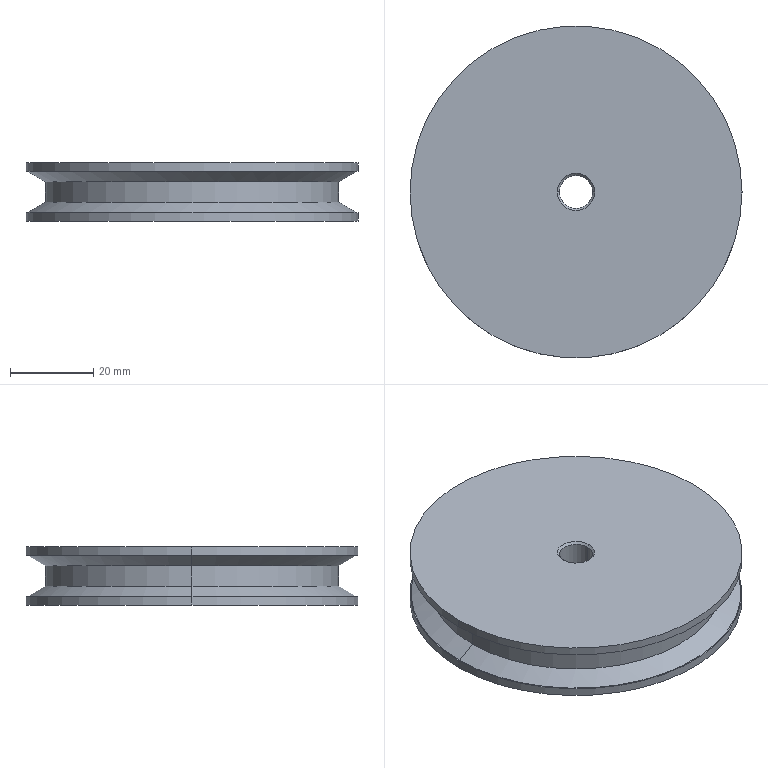Part | SolidWorks | features Chamfer 1, Extrusion 1, RevCut 1 | 1 solid | 20 faces | box 80 x 80 x 14 mm | volume 61206 mm3 | cone 8 | cylinder 8 | plane 4 | commonest cylinder face diameters 80 x4 8 x2 70.651 x2
STEP:
#1=CARTESIAN_POINT('',(4.,0.,-6.5));
#2=VERTEX_POINT('',#1);
#3=CARTESIAN_POINT('',(-4.,0.,-6.5));
#4=VERTEX_POINT('',#3);
#5=CARTESIAN_POINT('',(0.,0.,-6.5));
#6=DIRECTION('',(0.,0.,-1.));
#7=DIRECTION('',(1.,0.,0.));
#8=AXIS2_PLACEMENT_3D('',#5,#6,#7);
#9=CIRCLE('',#8,4.);
#10=EDGE_CURVE('',#2,#4,#9,.T.);
#11=ORIENTED_EDGE('',*,*,#10,.F.);
#12=CARTESIAN_POINT('',(4.5,0.,-7.));
#13=VERTEX_POINT('',#12);
#14=CARTESIAN_POINT('',(4.5,0.,-7.));
#15=DIRECTION('',(0.7071,0.,-0.7071));
#16=VECTOR('',#15,1000.);
#17=LINE('',#14,#16);
#18=EDGE_CURVE('',#2,#13,#17,.T.);
#19=ORIENTED_EDGE('',*,*,#18,.T.);
#20=CARTESIAN_POINT('',(-4.5,0.,-7.));
#21=VERTEX_POINT('',#20);
#22=CARTESIAN_POINT('',(0.,0.,-7.));
#23=DIRECTION('',(0.,0.,1.));
#24=DIRECTION('',(1.,0.,0.));
#25=AXIS2_PLACEMENT_3D('',#22,#23,#24);
#26=CIRCLE('',#25,4.5);
#27=EDGE_CURVE('',#21,#13,#26,.T.);
#28=ORIENTED_EDGE('',*,*,#27,.F.);
#29=CARTESIAN_POINT('',(-4.5,0.,-7.));
#30=DIRECTION('',(-0.7071,0.,-0.7071));
#31=VECTOR('',#30,1000.);
#32=LINE('',#29,#31);
#33=EDGE_CURVE('',#4,#21,#32,.T.);
#34=ORIENTED_EDGE('',*,*,#33,.F.);
#35=EDGE_LOOP('',(#11,#19,#28,#34));
#36=FACE_OUTER_BOUND('',#35,.T.);
#37=CARTESIAN_POINT('',(0.,0.,-7.));
#38=DIRECTION('',(0.,0.,-1.));
#39=DIRECTION('',(-1.,0.,0.));
#40=AXIS2_PLACEMENT_3D('',#37,#38,#39);
#41=CONICAL_SURFACE('',#40,4.5,0.7854);
#42=ADVANCED_FACE('',(#36),#41,.F.);
#43=CARTESIAN_POINT('',(-4.,0.,6.5));
#44=VERTEX_POINT('',#43);
#45=CARTESIAN_POINT('',(4.,0.,6.5));
#46=VERTEX_POINT('',#45);
#47=CARTESIAN_POINT('',(0.,0.,6.5));
#48=DIRECTION('',(0.,0.,1.));
#49=DIRECTION('',(1.,0.,0.));
#50=AXIS2_PLACEMENT_3D('',#47,#48,#49);
#51=CIRCLE('',#50,4.);
#52=EDGE_CURVE('',#44,#46,#51,.T.);
#53=ORIENTED_EDGE('',*,*,#52,.F.);
#54=CARTESIAN_POINT('',(-4.5,0.,7.));
#55=VERTEX_POINT('',#54);
#56=CARTESIAN_POINT('',(-4.,0.,6.5));
#57=DIRECTION('',(-0.7071,0.,0.7071));
#58=VECTOR('',#57,1000.);
#59=LINE('',#56,#58);
#60=EDGE_CURVE('',#44,#55,#59,.T.);
#61=ORIENTED_EDGE('',*,*,#60,.T.);
#62=CARTESIAN_POINT('',(4.5,0.,7.));
#63=VERTEX_POINT('',#62);
#64=CARTESIAN_POINT('',(0.,0.,7.));
#65=DIRECTION('',(0.,0.,-1.));
#66=DIRECTION('',(1.,0.,0.));
#67=AXIS2_PLACEMENT_3D('',#64,#65,#66);
#68=CIRCLE('',#67,4.5);
#69=EDGE_CURVE('',#63,#55,#68,.T.);
#70=ORIENTED_EDGE('',*,*,#69,.F.);
#71=CARTESIAN_POINT('',(4.,0.,6.5));
#72=DIRECTION('',(0.7071,0.,0.7071));
#73=VECTOR('',#72,1000.);
#74=LINE('',#71,#73);
#75=EDGE_CURVE('',#46,#63,#74,.T.);
#76=ORIENTED_EDGE('',*,*,#75,.F.);
#77=EDGE_LOOP('',(#53,#61,#70,#76));
#78=FACE_OUTER_BOUND('',#77,.T.);
#79=CARTESIAN_POINT('',(0.,0.,6.5));
#80=DIRECTION('',(0.,0.,1.));
#81=DIRECTION('',(1.,0.,0.));
#82=AXIS2_PLACEMENT_3D('',#79,#80,#81);
#83=CONICAL_SURFACE('',#82,4.,0.7854);
#84=ADVANCED_FACE('',(#78),#83,.F.);
#85=CARTESIAN_POINT('',(35.325,0.,-2.449));
#86=VERTEX_POINT('',#85);
#87=CARTESIAN_POINT('',(-35.325,0.,-2.449));
#88=VERTEX_POINT('',#87);
#89=CARTESIAN_POINT('',(0.,0.,-2.449));
#90=DIRECTION('',(0.,0.,1.));
#91=DIRECTION('',(1.,0.,0.));
#92=AXIS2_PLACEMENT_3D('',#89,#90,#91);
#93=CIRCLE('',#92,35.325);
#94=EDGE_CURVE('',#86,#88,#93,.T.);
#95=ORIENTED_EDGE('',*,*,#94,.F.);
#96=CARTESIAN_POINT('',(39.744,0.,-5.));
#97=VERTEX_POINT('',#96);
#98=CARTESIAN_POINT('',(35.325,0.,-2.449));
#99=DIRECTION('',(0.866,0.,-0.5));
#100=VECTOR('',#99,1000.);
#101=LINE('',#98,#100);
#102=EDGE_CURVE('',#86,#97,#101,.T.);
#103=ORIENTED_EDGE('',*,*,#102,.T.);
#104=CARTESIAN_POINT('',(-39.744,0.,-5.));
#105=VERTEX_POINT('',#104);
#106=CARTESIAN_POINT('',(0.,0.,-5.));
#107=DIRECTION('',(0.,0.,1.));
#108=DIRECTION('',(1.,0.,0.));
#109=AXIS2_PLACEMENT_3D('',#106,#107,#108);
#110=CIRCLE('',#109,39.744);
#111=EDGE_CURVE('',#97,#105,#110,.T.);
#112=ORIENTED_EDGE('',*,*,#111,.T.);
#113=CARTESIAN_POINT('',(-35.325,0.,-2.449));
#114=DIRECTION('',(-0.866,0.,-0.5));
#115=VECTOR('',#114,1000.);
#116=LINE('',#113,#115);
#117=EDGE_CURVE('',#88,#105,#116,.T.);
#118=ORIENTED_EDGE('',*,*,#117,.F.);
#119=EDGE_LOOP('',(#95,#103,#112,#118));
#120=FACE_OUTER_BOUND('',#119,.T.);
#121=CARTESIAN_POINT('',(0.,0.,-2.449));
#122=DIRECTION('',(0.,0.,-1.));
#123=DIRECTION('',(-1.,0.,0.));
#124=AXIS2_PLACEMENT_3D('',#121,#122,#123);
#125=CONICAL_SURFACE('',#124,35.325,1.047);
#126=ADVANCED_FACE('',(#120),#125,.T.);
#127=CARTESIAN_POINT('',(35.325,0.,2.449));
#128=VERTEX_POINT('',#127);
#129=CARTESIAN_POINT('',(-35.325,0.,2.449));
#130=VERTEX_POINT('',#129);
#131=CARTESIAN_POINT('',(0.,0.,2.449));
#132=DIRECTION('',(0.,0.,1.));
#133=DIRECTION('',(1.,0.,0.));
#134=AXIS2_PLACEMENT_3D('',#131,#132,#133);
#135=CIRCLE('',#134,35.325);
#136=EDGE_CURVE('',#128,#130,#135,.T.);
#137=ORIENTED_EDGE('',*,*,#136,.T.);
#138=CARTESIAN_POINT('',(-39.744,0.,5.));
#139=VERTEX_POINT('',#138);
#140=CARTESIAN_POINT('',(-39.744,0.,5.));
#141=DIRECTION('',(-0.866,0.,0.5));
#142=VECTOR('',#141,1000.);
#143=LINE('',#140,#142);
#144=EDGE_CURVE('',#130,#139,#143,.T.);
#145=ORIENTED_EDGE('',*,*,#144,.T.);
#146=CARTESIAN_POINT('',(39.744,0.,5.));
#147=VERTEX_POINT('',#146);
#148=CARTESIAN_POINT('',(0.,0.,5.));
#149=DIRECTION('',(0.,0.,1.));
#150=DIRECTION('',(1.,0.,0.));
#151=AXIS2_PLACEMENT_3D('',#148,#149,#150);
#152=CIRCLE('',#151,39.744);
#153=EDGE_CURVE('',#147,#139,#152,.T.);
#154=ORIENTED_EDGE('',*,*,#153,.F.);
#155=CARTESIAN_POINT('',(39.744,0.,5.));
#156=DIRECTION('',(0.866,0.,0.5));
#157=VECTOR('',#156,1000.);
#158=LINE('',#155,#157);
#159=EDGE_CURVE('',#128,#147,#158,.T.);
#160=ORIENTED_EDGE('',*,*,#159,.F.);
#161=EDGE_LOOP('',(#137,#145,#154,#160));
#162=FACE_OUTER_BOUND('',#161,.T.);
#163=CARTESIAN_POINT('',(0.,0.,5.));
#164=DIRECTION('',(0.,0.,1.));
#165=DIRECTION('',(1.,0.,0.));
#166=AXIS2_PLACEMENT_3D('',#163,#164,#165);
#167=CONICAL_SURFACE('',#166,39.744,1.047);
#168=ADVANCED_FACE('',(#162),#167,.T.);
#169=ORIENTED_EDGE('',*,*,#94,.T.);
#170=CARTESIAN_POINT('',(-35.325,0.,7.));
#171=DIRECTION('',(0.,0.,1.));
#172=VECTOR('',#171,1000.);
#173=LINE('',#170,#172);
#174=EDGE_CURVE('',#88,#130,#173,.T.);
#175=ORIENTED_EDGE('',*,*,#174,.T.);
#176=ORIENTED_EDGE('',*,*,#136,.F.);
#177=CARTESIAN_POINT('',(35.325,0.,7.));
#178=DIRECTION('',(0.,0.,1.));
#179=VECTOR('',#178,1000.);
#180=LINE('',#177,#179);
#181=EDGE_CURVE('',#86,#128,#180,.T.);
#182=ORIENTED_EDGE('',*,*,#181,.F.);
#183=EDGE_LOOP('',(#169,#175,#176,#182));
#184=FACE_OUTER_BOUND('',#183,.T.);
#185=CARTESIAN_POINT('',(0.,0.,7.));
#186=DIRECTION('',(0.,0.,1.));
#187=DIRECTION('',(1.,0.,0.));
#188=AXIS2_PLACEMENT_3D('',#185,#186,#187);
#189=CYLINDRICAL_SURFACE('',#188,35.325);
#190=ADVANCED_FACE('',(#184),#189,.T.);
#191=ORIENTED_EDGE('',*,*,#52,.T.);
#192=CARTESIAN_POINT('',(4.,0.,7.));
#193=DIRECTION('',(0.,0.,-1.));
#194=VECTOR('',#193,1000.);
#195=LINE('',#192,#194);
#196=EDGE_CURVE('',#46,#2,#195,.T.);
#197=ORIENTED_EDGE('',*,*,#196,.T.);
#198=ORIENTED_EDGE('',*,*,#10,.T.);
#199=CARTESIAN_POINT('',(-4.,0.,7.));
#200=DIRECTION('',(0.,0.,-1.));
#201=VECTOR('',#200,1000.);
#202=LINE('',#199,#201);
#203=EDGE_CURVE('',#44,#4,#202,.T.);
#204=ORIENTED_EDGE('',*,*,#203,.F.);
#205=EDGE_LOOP('',(#191,#197,#198,#204));
#206=FACE_OUTER_BOUND('',#205,.T.);
#207=CARTESIAN_POINT('',(0.,0.,7.));
#208=DIRECTION('',(0.,0.,-1.));
#209=DIRECTION('',(-1.,0.,0.));
#210=AXIS2_PLACEMENT_3D('',#207,#208,#209);
#211=CYLINDRICAL_SURFACE('',#210,4.);
#212=ADVANCED_FACE('',(#206),#211,.F.);
#213=CARTESIAN_POINT('',(40.,0.,-5.));
#214=VERTEX_POINT('',#213);
#215=CARTESIAN_POINT('',(-40.,0.,-5.));
#216=VERTEX_POINT('',#215);
#217=CARTESIAN_POINT('',(0.,0.,-5.));
#218=DIRECTION('',(0.,0.,1.));
#219=DIRECTION('',(1.,0.,0.));
#220=AXIS2_PLACEMENT_3D('',#217,#218,#219);
#221=CIRCLE('',#220,40.);
#222=EDGE_CURVE('',#214,#216,#221,.T.);
#223=ORIENTED_EDGE('',*,*,#222,.F.);
#224=CARTESIAN_POINT('',(40.,0.,-7.));
#225=VERTEX_POINT('',#224);
#226=CARTESIAN_POINT('',(40.,0.,7.));
#227=DIRECTION('',(0.,0.,-1.));
#228=VECTOR('',#227,1000.);
#229=LINE('',#226,#228);
#230=EDGE_CURVE('',#214,#225,#229,.T.);
#231=ORIENTED_EDGE('',*,*,#230,.T.);
#232=CARTESIAN_POINT('',(-40.,0.,-7.));
#233=VERTEX_POINT('',#232);
#234=CARTESIAN_POINT('',(0.,0.,-7.));
#235=DIRECTION('',(0.,0.,1.));
#236=DIRECTION('',(1.,0.,0.));
#237=AXIS2_PLACEMENT_3D('',#234,#235,#236);
#238=CIRCLE('',#237,40.);
#239=EDGE_CURVE('',#225,#233,#238,.T.);
#240=ORIENTED_EDGE('',*,*,#239,.T.);
#241=CARTESIAN_POINT('',(-40.,0.,7.));
#242=DIRECTION('',(0.,0.,-1.));
#243=VECTOR('',#242,1000.);
#244=LINE('',#241,#243);
#245=EDGE_CURVE('',#216,#233,#244,.T.);
#246=ORIENTED_EDGE('',*,*,#245,.F.);
#247=EDGE_LOOP('',(#223,#231,#240,#246));
#248=FACE_OUTER_BOUND('',#247,.T.);
#249=CARTESIAN_POINT('',(0.,0.,7.));
#250=DIRECTION('',(0.,0.,-1.));
#251=DIRECTION('',(-1.,0.,0.));
#252=AXIS2_PLACEMENT_3D('',#249,#250,#251);
#253=CYLINDRICAL_SURFACE('',#252,40.);
#254=ADVANCED_FACE('',(#248),#253,.T.);
#255=CARTESIAN_POINT('',(40.,0.,7.));
#256=VERTEX_POINT('',#255);
#257=CARTESIAN_POINT('',(-40.,0.,7.));
#258=VERTEX_POINT('',#257);
#259=CARTESIAN_POINT('',(0.,0.,7.));
#260=DIRECTION('',(0.,0.,1.));
#261=DIRECTION('',(1.,0.,0.));
#262=AXIS2_PLACEMENT_3D('',#259,#260,#261);
#263=CIRCLE('',#262,40.);
#264=EDGE_CURVE('',#256,#258,#263,.T.);
#265=ORIENTED_EDGE('',*,*,#264,.F.);
#266=CARTESIAN_POINT('',(40.,0.,5.));
#267=VERTEX_POINT('',#266);
#268=CARTESIAN_POINT('',(40.,0.,7.));
#269=DIRECTION('',(0.,0.,-1.));
#270=VECTOR('',#269,1000.);
#271=LINE('',#268,#270);
#272=EDGE_CURVE('',#256,#267,#271,.T.);
#273=ORIENTED_EDGE('',*,*,#272,.T.);
#274=CARTESIAN_POINT('',(-40.,0.,5.));
#275=VERTEX_POINT('',#274);
#276=CARTESIAN_POINT('',(0.,0.,5.));
#277=DIRECTION('',(0.,0.,1.));
#278=DIRECTION('',(1.,0.,0.));
#279=AXIS2_PLACEMENT_3D('',#276,#277,#278);
#280=CIRCLE('',#279,40.);
#281=EDGE_CURVE('',#267,#275,#280,.T.);
#282=ORIENTED_EDGE('',*,*,#281,.T.);
#283=CARTESIAN_POINT('',(-40.,0.,7.));
#284=DIRECTION('',(0.,0.,-1.));
#285=VECTOR('',#284,1000.);
#286=LINE('',#283,#285);
#287=EDGE_CURVE('',#258,#275,#286,.T.);
#288=ORIENTED_EDGE('',*,*,#287,.F.);
#289=EDGE_LOOP('',(#265,#273,#282,#288));
#290=FACE_OUTER_BOUND('',#289,.T.);
#291=CARTESIAN_POINT('',(0.,0.,7.));
#292=DIRECTION('',(0.,0.,-1.));
#293=DIRECTION('',(-1.,0.,0.));
#294=AXIS2_PLACEMENT_3D('',#291,#292,#293);
#295=CYLINDRICAL_SURFACE('',#294,40.);
#296=ADVANCED_FACE('',(#290),#295,.T.);
#297=ORIENTED_EDGE('',*,*,#272,.F.);
#298=CARTESIAN_POINT('',(0.,0.,7.));
#299=DIRECTION('',(0.,0.,1.));
#300=DIRECTION('',(1.,0.,0.));
#301=AXIS2_PLACEMENT_3D('',#298,#299,#300);
#302=CIRCLE('',#301,40.);
#303=EDGE_CURVE('',#258,#256,#302,.T.);
#304=ORIENTED_EDGE('',*,*,#303,.F.);
#305=ORIENTED_EDGE('',*,*,#287,.T.);
#306=CARTESIAN_POINT('',(0.,0.,5.));
#307=DIRECTION('',(0.,0.,1.));
#308=DIRECTION('',(1.,0.,0.));
#309=AXIS2_PLACEMENT_3D('',#306,#307,#308);
#310=CIRCLE('',#309,40.);
#311=EDGE_CURVE('',#275,#267,#310,.T.);
#312=ORIENTED_EDGE('',*,*,#311,.T.);
#313=EDGE_LOOP('',(#297,#304,#305,#312));
#314=FACE_OUTER_BOUND('',#313,.T.);
#315=CARTESIAN_POINT('',(0.,0.,7.));
#316=DIRECTION('',(0.,0.,-1.));
#317=DIRECTION('',(-1.,0.,0.));
#318=AXIS2_PLACEMENT_3D('',#315,#316,#317);
#319=CYLINDRICAL_SURFACE('',#318,40.);
#320=ADVANCED_FACE('',(#314),#319,.T.);
#321=ORIENTED_EDGE('',*,*,#230,.F.);
#322=CARTESIAN_POINT('',(0.,0.,-5.));
#323=DIRECTION('',(0.,0.,1.));
#324=DIRECTION('',(1.,0.,0.));
#325=AXIS2_PLACEMENT_3D('',#322,#323,#324);
#326=CIRCLE('',#325,40.);
#327=EDGE_CURVE('',#216,#214,#326,.T.);
#328=ORIENTED_EDGE('',*,*,#327,.F.);
#329=ORIENTED_EDGE('',*,*,#245,.T.);
#330=CARTESIAN_POINT('',(0.,0.,-7.));
#331=DIRECTION('',(0.,0.,1.));
#332=DIRECTION('',(1.,0.,0.));
#333=AXIS2_PLACEMENT_3D('',#330,#331,#332);
#334=CIRCLE('',#333,40.);
#335=EDGE_CURVE('',#233,#225,#334,.T.);
#336=ORIENTED_EDGE('',*,*,#335,.T.);
#337=EDGE_LOOP('',(#321,#328,#329,#336));
#338=FACE_OUTER_BOUND('',#337,.T.);
#339=CARTESIAN_POINT('',(0.,0.,7.));
#340=DIRECTION('',(0.,0.,-1.));
#341=DIRECTION('',(-1.,0.,0.));
#342=AXIS2_PLACEMENT_3D('',#339,#340,#341);
#343=CYLINDRICAL_SURFACE('',#342,40.);
#344=ADVANCED_FACE('',(#338),#343,.T.);
#345=ORIENTED_EDGE('',*,*,#69,.T.);
#346=CARTESIAN_POINT('',(0.,0.,7.));
#347=DIRECTION('',(0.,0.,-1.));
#348=DIRECTION('',(1.,0.,0.));
#349=AXIS2_PLACEMENT_3D('',#346,#347,#348);
#350=CIRCLE('',#349,4.5);
#351=EDGE_CURVE('',#55,#63,#350,.T.);
#352=ORIENTED_EDGE('',*,*,#351,.T.);
#353=EDGE_LOOP('',(#345,#352));
#354=FACE_BOUND('',#353,.T.);
#355=ORIENTED_EDGE('',*,*,#303,.T.);
#356=ORIENTED_EDGE('',*,*,#264,.T.);
#357=EDGE_LOOP('',(#355,#356));
#358=FACE_OUTER_BOUND('',#357,.T.);
#359=CARTESIAN_POINT('',(0.,0.,7.));
#360=DIRECTION('',(0.,0.,1.));
#361=DIRECTION('',(1.,0.,0.));
#362=AXIS2_PLACEMENT_3D('',#359,#360,#361);
#363=PLANE('',#362);
#364=ADVANCED_FACE('',(#354,#358),#363,.T.);
#365=ORIENTED_EDGE('',*,*,#27,.T.);
#366=CARTESIAN_POINT('',(0.,0.,-7.));
#367=DIRECTION('',(0.,0.,1.));
#368=DIRECTION('',(1.,0.,0.));
#369=AXIS2_PLACEMENT_3D('',#366,#367,#368);
#370=CIRCLE('',#369,4.5);
#371=EDGE_CURVE('',#13,#21,#370,.T.);
#372=ORIENTED_EDGE('',*,*,#371,.T.);
#373=EDGE_LOOP('',(#365,#372));
#374=FACE_BOUND('',#373,.T.);
#375=ORIENTED_EDGE('',*,*,#335,.F.);
#376=ORIENTED_EDGE('',*,*,#239,.F.);
#377=EDGE_LOOP('',(#375,#376));
#378=FACE_OUTER_BOUND('',#377,.T.);
#379=CARTESIAN_POINT('',(0.,0.,-7.));
#380=DIRECTION('',(0.,0.,1.));
#381=DIRECTION('',(1.,0.,0.));
#382=AXIS2_PLACEMENT_3D('',#379,#380,#381);
#383=PLANE('',#382);
#384=ADVANCED_FACE('',(#374,#378),#383,.F.);
#385=ORIENTED_EDGE('',*,*,#196,.F.);
#386=CARTESIAN_POINT('',(0.,0.,6.5));
#387=DIRECTION('',(0.,0.,1.));
#388=DIRECTION('',(1.,0.,0.));
#389=AXIS2_PLACEMENT_3D('',#386,#387,#388);
#390=CIRCLE('',#389,4.);
#391=EDGE_CURVE('',#46,#44,#390,.T.);
#392=ORIENTED_EDGE('',*,*,#391,.T.);
#393=ORIENTED_EDGE('',*,*,#203,.T.);
#394=CARTESIAN_POINT('',(0.,0.,-6.5));
#395=DIRECTION('',(0.,0.,-1.));
#396=DIRECTION('',(1.,0.,0.));
#397=AXIS2_PLACEMENT_3D('',#394,#395,#396);
#398=CIRCLE('',#397,4.);
#399=EDGE_CURVE('',#4,#2,#398,.T.);
#400=ORIENTED_EDGE('',*,*,#399,.T.);
#401=EDGE_LOOP('',(#385,#392,#393,#400));
#402=FACE_OUTER_BOUND('',#401,.T.);
#403=CARTESIAN_POINT('',(0.,0.,7.));
#404=DIRECTION('',(0.,0.,-1.));
#405=DIRECTION('',(-1.,0.,0.));
#406=AXIS2_PLACEMENT_3D('',#403,#404,#405);
#407=CYLINDRICAL_SURFACE('',#406,4.);
#408=ADVANCED_FACE('',(#402),#407,.F.);
#409=ORIENTED_EDGE('',*,*,#174,.F.);
#410=CARTESIAN_POINT('',(0.,0.,-2.449));
#411=DIRECTION('',(0.,0.,1.));
#412=DIRECTION('',(1.,0.,0.));
#413=AXIS2_PLACEMENT_3D('',#410,#411,#412);
#414=CIRCLE('',#413,35.325);
#415=EDGE_CURVE('',#88,#86,#414,.T.);
#416=ORIENTED_EDGE('',*,*,#415,.T.);
#417=ORIENTED_EDGE('',*,*,#181,.T.);
#418=CARTESIAN_POINT('',(0.,0.,2.449));
#419=DIRECTION('',(0.,0.,1.));
#420=DIRECTION('',(1.,0.,0.));
#421=AXIS2_PLACEMENT_3D('',#418,#419,#420);
#422=CIRCLE('',#421,35.325);
#423=EDGE_CURVE('',#130,#128,#422,.T.);
#424=ORIENTED_EDGE('',*,*,#423,.F.);
#425=EDGE_LOOP('',(#409,#416,#417,#424));
#426=FACE_OUTER_BOUND('',#425,.T.);
#427=CARTESIAN_POINT('',(0.,0.,7.));
#428=DIRECTION('',(0.,0.,1.));
#429=DIRECTION('',(1.,0.,0.));
#430=AXIS2_PLACEMENT_3D('',#427,#428,#429);
#431=CYLINDRICAL_SURFACE('',#430,35.325);
#432=ADVANCED_FACE('',(#426),#431,.T.);
#433=ORIENTED_EDGE('',*,*,#144,.F.);
#434=ORIENTED_EDGE('',*,*,#423,.T.);
#435=ORIENTED_EDGE('',*,*,#159,.T.);
#436=CARTESIAN_POINT('',(0.,0.,5.));
#437=DIRECTION('',(0.,0.,1.));
#438=DIRECTION('',(1.,0.,0.));
#439=AXIS2_PLACEMENT_3D('',#436,#437,#438);
#440=CIRCLE('',#439,39.744);
#441=EDGE_CURVE('',#139,#147,#440,.T.);
#442=ORIENTED_EDGE('',*,*,#441,.F.);
#443=EDGE_LOOP('',(#433,#434,#435,#442));
#444=FACE_OUTER_BOUND('',#443,.T.);
#445=CARTESIAN_POINT('',(0.,0.,5.));
#446=DIRECTION('',(0.,0.,1.));
#447=DIRECTION('',(1.,0.,0.));
#448=AXIS2_PLACEMENT_3D('',#445,#446,#447);
#449=CONICAL_SURFACE('',#448,39.744,1.047);
#450=ADVANCED_FACE('',(#444),#449,.T.);
#451=ORIENTED_EDGE('',*,*,#153,.T.);
#452=ORIENTED_EDGE('',*,*,#441,.T.);
#453=EDGE_LOOP('',(#451,#452));
#454=FACE_BOUND('',#453,.T.);
#455=ORIENTED_EDGE('',*,*,#311,.F.);
#456=ORIENTED_EDGE('',*,*,#281,.F.);
#457=EDGE_LOOP('',(#455,#456));
#458=FACE_OUTER_BOUND('',#457,.T.);
#459=CARTESIAN_POINT('',(0.,40.,5.));
#460=DIRECTION('',(0.,0.,-1.));
#461=DIRECTION('',(-1.,0.,0.));
#462=AXIS2_PLACEMENT_3D('',#459,#460,#461);
#463=PLANE('',#462);
#464=ADVANCED_FACE('',(#454,#458),#463,.T.);
#465=ORIENTED_EDGE('',*,*,#327,.T.);
#466=ORIENTED_EDGE('',*,*,#222,.T.);
#467=EDGE_LOOP('',(#465,#466));
#468=FACE_OUTER_BOUND('',#467,.T.);
#469=CARTESIAN_POINT('',(0.,0.,-5.));
#470=DIRECTION('',(0.,0.,1.));
#471=DIRECTION('',(1.,0.,0.));
#472=AXIS2_PLACEMENT_3D('',#469,#470,#471);
#473=CIRCLE('',#472,39.744);
#474=EDGE_CURVE('',#105,#97,#473,.T.);
#475=ORIENTED_EDGE('',*,*,#474,.F.);
#476=ORIENTED_EDGE('',*,*,#111,.F.);
#477=EDGE_LOOP('',(#475,#476));
#478=FACE_BOUND('',#477,.T.);
#479=CARTESIAN_POINT('',(0.,40.,-5.));
#480=DIRECTION('',(0.,0.,1.));
#481=DIRECTION('',(1.,0.,0.));
#482=AXIS2_PLACEMENT_3D('',#479,#480,#481);
#483=PLANE('',#482);
#484=ADVANCED_FACE('',(#468,#478),#483,.T.);
#485=ORIENTED_EDGE('',*,*,#102,.F.);
#486=ORIENTED_EDGE('',*,*,#415,.F.);
#487=ORIENTED_EDGE('',*,*,#117,.T.);
#488=ORIENTED_EDGE('',*,*,#474,.T.);
#489=EDGE_LOOP('',(#485,#486,#487,#488));
#490=FACE_OUTER_BOUND('',#489,.T.);
#491=CARTESIAN_POINT('',(0.,0.,-2.449));
#492=DIRECTION('',(0.,0.,-1.));
#493=DIRECTION('',(-1.,0.,0.));
#494=AXIS2_PLACEMENT_3D('',#491,#492,#493);
#495=CONICAL_SURFACE('',#494,35.325,1.047);
#496=ADVANCED_FACE('',(#490),#495,.T.);
#497=ORIENTED_EDGE('',*,*,#60,.F.);
#498=ORIENTED_EDGE('',*,*,#391,.F.);
#499=ORIENTED_EDGE('',*,*,#75,.T.);
#500=ORIENTED_EDGE('',*,*,#351,.F.);
#501=EDGE_LOOP('',(#497,#498,#499,#500));
#502=FACE_OUTER_BOUND('',#501,.T.);
#503=CARTESIAN_POINT('',(0.,0.,6.5));
#504=DIRECTION('',(0.,0.,1.));
#505=DIRECTION('',(1.,0.,0.));
#506=AXIS2_PLACEMENT_3D('',#503,#504,#505);
#507=CONICAL_SURFACE('',#506,4.,0.7854);
#508=ADVANCED_FACE('',(#502),#507,.F.);
#509=ORIENTED_EDGE('',*,*,#18,.F.);
#510=ORIENTED_EDGE('',*,*,#399,.F.);
#511=ORIENTED_EDGE('',*,*,#33,.T.);
#512=ORIENTED_EDGE('',*,*,#371,.F.);
#513=EDGE_LOOP('',(#509,#510,#511,#512));
#514=FACE_OUTER_BOUND('',#513,.T.);
#515=CARTESIAN_POINT('',(0.,0.,-7.));
#516=DIRECTION('',(0.,0.,-1.));
#517=DIRECTION('',(-1.,0.,0.));
#518=AXIS2_PLACEMENT_3D('',#515,#516,#517);
#519=CONICAL_SURFACE('',#518,4.5,0.7854);
#520=ADVANCED_FACE('',(#514),#519,.F.);
#521=CLOSED_SHELL('',(#42,#84,#126,#168,#190,#212,#254,#296,#320,#344,#364,#384,#408,#432,#450,#464,#484,#496,#508,#520));
#522=MANIFOLD_SOLID_BREP('',#521);
#523=CARTESIAN_POINT('',(0.,0.,0.));
#524=DIRECTION('',(0.,0.,1.));
#525=DIRECTION('',(1.,0.,0.));
#526=AXIS2_PLACEMENT_3D('',#523,#524,#525);
#527=(LENGTH_UNIT()NAMED_UNIT(*)SI_UNIT(.MILLI.,.METRE.));
#528=UNCERTAINTY_MEASURE_WITH_UNIT(LENGTH_MEASURE(0.00001),#527,'','');
#529=(NAMED_UNIT(*)PLANE_ANGLE_UNIT()SI_UNIT($,.RADIAN.));
#530=(NAMED_UNIT(*)SI_UNIT($,.STERADIAN.)SOLID_ANGLE_UNIT());
#531=(GEOMETRIC_REPRESENTATION_CONTEXT(3)GLOBAL_UNCERTAINTY_ASSIGNED_CONTEXT((#528))GLOBAL_UNIT_ASSIGNED_CONTEXT((#527,#529,#530))REPRESENTATION_CONTEXT('',''));
#532=ADVANCED_BREP_SHAPE_REPRESENTATION('',(#522,#526),#531);